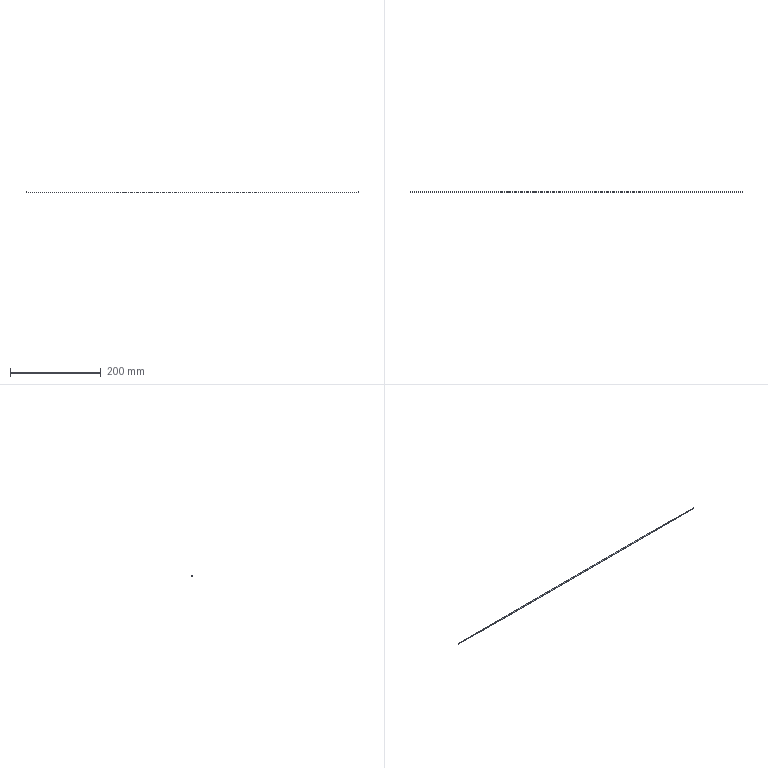Part | NX | 1 solid | 4 faces | box 730 x 2 x 2 mm | volume 2293 mm3 | cylinder 2 | plane 2 | commonest cylinder face diameters 2 x2
STEP:
#1=CARTESIAN_POINT('',(640.,208.2,-31.5));
#2=VERTEX_POINT('',#1);
#3=CARTESIAN_POINT('',(640.,210.2,-31.5));
#4=VERTEX_POINT('',#3);
#5=CARTESIAN_POINT('',(640.,209.2,-31.5));
#6=DIRECTION('',(-1.,0.,0.));
#7=DIRECTION('',(0.,-1.,0.));
#8=AXIS2_PLACEMENT_3D('',#5,#6,#7);
#9=CIRCLE('',#8,1.);
#10=EDGE_CURVE('',#2,#4,#9,.T.);
#11=ORIENTED_EDGE('',*,*,#10,.T.);
#12=CARTESIAN_POINT('',(-90.,210.2,-31.5));
#13=VERTEX_POINT('',#12);
#14=CARTESIAN_POINT('',(-140.,210.2,-31.5));
#15=DIRECTION('',(-1.,0.,0.));
#16=VECTOR('',#15,1000.);
#17=LINE('',#14,#16);
#18=EDGE_CURVE('',#13,#4,#17,.F.);
#19=ORIENTED_EDGE('',*,*,#18,.F.);
#20=CARTESIAN_POINT('',(-90.,208.2,-31.5));
#21=VERTEX_POINT('',#20);
#22=CARTESIAN_POINT('',(-90.,209.2,-31.5));
#23=DIRECTION('',(-1.,0.,0.));
#24=DIRECTION('',(0.,-1.,0.));
#25=AXIS2_PLACEMENT_3D('',#22,#23,#24);
#26=CIRCLE('',#25,1.);
#27=EDGE_CURVE('',#21,#13,#26,.T.);
#28=ORIENTED_EDGE('',*,*,#27,.F.);
#29=CARTESIAN_POINT('',(-140.,208.2,-31.5));
#30=DIRECTION('',(-1.,0.,0.));
#31=VECTOR('',#30,1000.);
#32=LINE('',#29,#31);
#33=EDGE_CURVE('',#21,#2,#32,.F.);
#34=ORIENTED_EDGE('',*,*,#33,.T.);
#35=EDGE_LOOP('',(#11,#19,#28,#34));
#36=FACE_BOUND('',#35,.T.);
#37=CARTESIAN_POINT('',(-140.,209.2,-31.5));
#38=DIRECTION('',(-1.,0.,0.));
#39=DIRECTION('',(0.,-1.,0.));
#40=AXIS2_PLACEMENT_3D('',#37,#38,#39);
#41=CYLINDRICAL_SURFACE('',#40,1.);
#42=ADVANCED_FACE('',(#36),#41,.T.);
#43=ORIENTED_EDGE('',*,*,#27,.T.);
#44=CARTESIAN_POINT('',(-90.,209.2,-31.5));
#45=DIRECTION('',(-1.,0.,0.));
#46=DIRECTION('',(0.,-1.,0.));
#47=AXIS2_PLACEMENT_3D('',#44,#45,#46);
#48=CIRCLE('',#47,1.);
#49=EDGE_CURVE('',#13,#21,#48,.T.);
#50=ORIENTED_EDGE('',*,*,#49,.T.);
#51=EDGE_LOOP('',(#43,#50));
#52=FACE_BOUND('',#51,.T.);
#53=CARTESIAN_POINT('',(-90.,205.822,-46.315));
#54=DIRECTION('',(-1.,0.,0.));
#55=DIRECTION('',(0.,0.,1.));
#56=AXIS2_PLACEMENT_3D('',#53,#54,#55);
#57=PLANE('',#56);
#58=ADVANCED_FACE('',(#52),#57,.T.);
#59=ORIENTED_EDGE('',*,*,#10,.F.);
#60=CARTESIAN_POINT('',(640.,209.2,-31.5));
#61=DIRECTION('',(-1.,0.,0.));
#62=DIRECTION('',(0.,-1.,0.));
#63=AXIS2_PLACEMENT_3D('',#60,#61,#62);
#64=CIRCLE('',#63,1.);
#65=EDGE_CURVE('',#4,#2,#64,.T.);
#66=ORIENTED_EDGE('',*,*,#65,.F.);
#67=EDGE_LOOP('',(#59,#66));
#68=FACE_BOUND('',#67,.T.);
#69=CARTESIAN_POINT('',(640.,205.822,-46.315));
#70=DIRECTION('',(-1.,0.,0.));
#71=DIRECTION('',(0.,0.,1.));
#72=AXIS2_PLACEMENT_3D('',#69,#70,#71);
#73=PLANE('',#72);
#74=ADVANCED_FACE('',(#68),#73,.F.);
#75=ORIENTED_EDGE('',*,*,#33,.F.);
#76=ORIENTED_EDGE('',*,*,#49,.F.);
#77=ORIENTED_EDGE('',*,*,#18,.T.);
#78=ORIENTED_EDGE('',*,*,#65,.T.);
#79=EDGE_LOOP('',(#75,#76,#77,#78));
#80=FACE_BOUND('',#79,.T.);
#81=CARTESIAN_POINT('',(-140.,209.2,-31.5));
#82=DIRECTION('',(-1.,0.,0.));
#83=DIRECTION('',(0.,-1.,0.));
#84=AXIS2_PLACEMENT_3D('',#81,#82,#83);
#85=CYLINDRICAL_SURFACE('',#84,1.);
#86=ADVANCED_FACE('',(#80),#85,.T.);
#87=CLOSED_SHELL('',(#42,#58,#74,#86));
#88=MANIFOLD_SOLID_BREP('',#87);
#89=(LENGTH_UNIT()NAMED_UNIT(*)SI_UNIT(.MILLI.,.METRE.));
#90=UNCERTAINTY_MEASURE_WITH_UNIT(LENGTH_MEASURE(0.00001),#89,'','');
#91=(NAMED_UNIT(*)PLANE_ANGLE_UNIT()SI_UNIT($,.RADIAN.));
#92=(NAMED_UNIT(*)SI_UNIT($,.STERADIAN.)SOLID_ANGLE_UNIT());
#93=(GEOMETRIC_REPRESENTATION_CONTEXT(3)GLOBAL_UNCERTAINTY_ASSIGNED_CONTEXT((#90))GLOBAL_UNIT_ASSIGNED_CONTEXT((#89,#91,#92))REPRESENTATION_CONTEXT('',''));
#94=ADVANCED_BREP_SHAPE_REPRESENTATION('',(#88),#93);